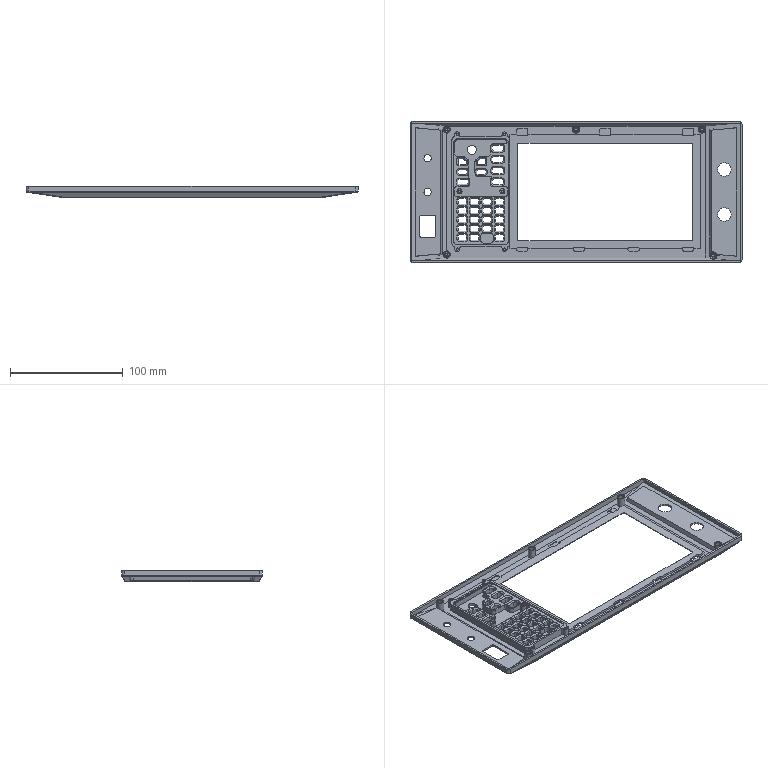NC program | NX | posted with a generic post | part box 295 x 125 x 10 mm
Lines 5491 to 6455 of 134431:
(CAVITY_MILL_COPY , TOOL : D6)
N10944 T06 M6
N10946 G54
N10948 G17 G0 G90 X112.278 Y-56.8 S9500 M3
N10950 G43 Z30. H6
N10952 Z0.5
N10954 G94 G1 Z-0.5 F1000.
N10956 X112.683 Y-57.5
N10958 G3 X113.549 Y-58. R1.
N10960 G1 X115.933 F2000.
N10962 G2 X115.782 Y-55.868 R6.25
N10964 G3 X115.372 Y-54.956 R1.
N10966 G1 X114.81 Y-54.55
N10968 Z0.5
N10970 G0 Z30.
N10972 X112.278 Y-56.8
N10974 Z0.
N10976 G1 Z-1. F1000.
N10978 X112.683 Y-57.5
N10980 G3 X113.549 Y-58. R1.
N10982 G1 X115.933 F2000.
N10984 G2 X115.782 Y-55.869 R6.25
N10986 G3 X115.372 Y-54.956 R1.
N10988 G1 X114.81 Y-54.551
N10990 Z0.
N10992 G0 X112.278 Y-56.8 Z-0.5
N10994 G1 Z-1.5 F1000.
N10996 X112.682 Y-57.5
N10998 G3 X113.548 Y-58. R1.
N11000 G1 X115.933 F2000.
N11002 G2 X115.782 Y-55.869 R6.25
N11004 G3 X115.372 Y-54.956 R1.
N11006 G1 X114.81 Y-54.551
N11008 Z-0.5
N11010 G0 X112.278 Y-56.8 Z-1.
N11012 G1 Z-2. F1000.
N11014 X112.682 Y-57.5
N11016 G3 X113.548 Y-58. R1.
N11018 G1 X115.933 F2000.
N11020 G2 X115.782 Y-55.868 R6.25
N11022 G3 X115.372 Y-54.956 R1.
N11024 G1 X114.81 Y-54.551
N11026 Z-1.
N11028 G0 X112.278 Y-56.8 Z-1.5
N11030 G1 Z-2.5 F1000.
N11032 X112.682 Y-57.5
N11034 G3 X113.548 Y-58. R1.
N11036 G1 X115.933 F2000.
N11038 G2 X115.782 Y-55.868 R6.25
N11040 G3 X115.372 Y-54.956 R1.
N11042 G1 X114.81 Y-54.551
N11044 Z-1.5
N11046 G0 X112.278 Y-56.8 Z-2.
N11048 G1 Z-3. F1000.
N11050 X112.682 Y-57.5
N11052 G3 X113.548 Y-58. R1.
N11054 G1 X115.933 F2000.
N11056 G2 X115.782 Y-55.868 R6.25
N11058 G3 X115.372 Y-54.956 R1.
N11060 G1 X114.81 Y-54.55
N11062 Z-2.
N11064 G0 X112.278 Y-56.8 Z-2.5
N11066 G1 Z-3.5 F1000.
N11068 X112.682 Y-57.5
N11070 G3 X113.548 Y-58. R1.
N11072 G1 X115.933 F2000.
N11074 G2 X115.782 Y-55.868 R6.25
N11076 G3 X115.372 Y-54.956 R1.
N11078 G1 X114.81 Y-54.55
N11080 Z-2.5
N11082 G0 X112.278 Y-56.8 Z-2.885
N11084 G1 Z-3.885 F1000.
N11086 X112.682 Y-57.5
N11088 G3 X113.548 Y-58. R1.
N11090 G1 X115.933 F2000.
N11092 G2 X115.782 Y-55.868 R6.25
N11094 G3 X115.372 Y-54.956 R1.
N11096 G1 X114.81 Y-54.55
N11098 Z-2.885
N11100 G0 X112.278 Y-56.8 Z-3.269
N11102 G1 Z-4.269 F1000.
N11104 X112.682 Y-57.5
N11106 G3 X113.548 Y-58. R1.
N11108 G1 X115.933 F2000.
N11110 G2 X115.782 Y-55.868 R6.25
N11112 G3 X115.372 Y-54.956 R1.
N11114 G1 X114.81 Y-54.55
N11116 Z-3.269
N11118 G0 X112.289 Y-56.655 Z-3.827
N11120 G1 Z-4.827 F1000.
N11122 X112.693 Y-57.355
N11124 G3 X113.559 Y-57.855 R1.
N11126 G1 X115.899 F2000.
N11128 G2 X115.794 Y-55.759 R6.25
N11130 G3 X115.4 Y-54.84 R1.
N11132 G1 X114.845 Y-54.424
N11134 Z-3.827
N11136 G0 X112.322 Y-56.32 Z-4.385
N11138 G1 Z-5.385 F1000.
N11140 X112.726 Y-57.02
N11142 G3 X113.592 Y-57.52 R1.
N11144 G1 X115.834 F2000.
N11146 G2 X115.829 Y-55.507 R6.25
N11148 G3 X115.473 Y-54.572 R1.
N11150 G1 X114.936 Y-54.134
N11152 Z-4.385
N11154 G0 X112.369 Y-55.985 Z-4.942
N11156 G1 Z-5.942 F1000.
N11158 X112.773 Y-56.685
N11160 G3 X113.639 Y-57.185 R1.
N11162 G1 X115.788 F2000.
N11164 G2 X115.875 Y-55.255 R6.25
N11166 G3 X115.558 Y-54.307 R1.
N11168 G1 X114.754 Y-53.595
N11170 Z-4.942
N11172 G0 X112.43 Y-55.652 Z-5.5
N11174 G1 Z-6.5 F1000.
N11176 X112.834 Y-56.352
N11178 G3 X113.7 Y-56.852 R1.
N11180 G1 X115.76 F2000.
N11182 G2 X115.932 Y-55.005 R6.25
N11184 G3 X115.653 Y-54.044 R1.
N11186 G1 X114.743 Y-53.17
N11188 Z-5.5
N11190 G0 X113.114 Y-54.608 Z-6.
N11192 G1 Z-7. F1000.
N11194 X112.113 Y-54.791
N11196 G2 X112.113 Y-53.791 R1.
N11198 X112.421 Y-53.413 R1.52 F2000.
N11200 G3 X112.495 Y-52.746 R0.5
N11202 G2 X110.54 Y-53.47 R3.
N11204 G1 X104.54
N11206 G2 X101.942 Y-51.97 R3.
N11208 G1 X100.753
N11210 G3 X101.183 Y-52.465 R0.5
N11212 G2 X101.933 Y-52.794 R1.52
N11214 G3 X102.545 Y-52.811 R0.5
N11216 X102.659 Y-53.413 R0.5
N11218 G2 X101.864 Y-56.056 R1.52
N11220 G3 X101.434 Y-56.551 R0.5
N11222 G1 X113.646
N11224 G3 X113.216 Y-56.056 R0.5
N11226 G2 X112.113 Y-53.791 R1.52
N11228 X112.979 Y-53.291 R1.
N11230 G1 X113.537 Y-53.931
N11232 Z-6.
N11234 G0 Z30.
N11236 X114.915 Y-54.198
N11238 Z-3.827
N11240 G1 Z-4.827 F1000.
N11242 X115.607 Y-54.166
N11244 G3 X116.45 Y-53.627 R1.
N11246 G2 X116.833 Y-52.983 R6.25 F2000.
N11248 G1 Y-52.197
N11250 G3 X116.333 Y-51.331 R1.
N11252 G1 X115.633 Y-50.927
N11254 Z-3.827
N11256 G0 X114.833 Y-54.467 Z-4.385
N11258 G1 Z-5.385 F1000.
N11260 X115.524 Y-54.409
N11262 G3 X116.345 Y-53.839 R1.
N11264 G2 X116.684 Y-53.214 R6.25 F2000.
N11266 G1 Y-52.471
N11268 G3 X116.184 Y-51.605 R1.
N11270 G1 X115.484 Y-51.201
N11272 Z-4.385
N11274 G0 X114.379 Y-54.809 Z-4.942
N11276 G1 Z-5.942 F1000.
N11278 X115.444 Y-54.675
N11280 G3 X116.241 Y-54.072 R1.
N11282 G2 X116.534 Y-53.469 R6.25 F2000.
N11284 G1 Y-52.773
N11286 G3 X116.034 Y-51.907 R1.
N11288 G1 X115.334 Y-51.502
N11290 Z-4.942
N11292 G0 X113.559 Y-55.278 Z-5.5
N11294 G1 Z-6.5 F1000.
N11296 X115.369 Y-54.969
N11298 G3 X116.139 Y-54.33 R1.
N11300 G2 X116.386 Y-53.754 R6.25 F2000.
N11302 G1 Y-53.108
N11304 G3 X115.886 Y-52.242 R1.
N11306 G1 X115.186 Y-51.838
N11308 Z-5.5
N11310 G0 Z30.
N11312 X129.191 Y-54.551
N11314 Z0.5
N11316 G1 Z-0.5 F1000.
N11318 X128.628 Y-54.957
N11320 G3 X128.218 Y-55.869 R1.
N11322 G2 X128.067 Y-58. R6.25 F2000.
N11324 G1 X130.451
N11326 G3 X131.317 Y-57.5 R1.
N11328 G1 X131.722 Y-56.8
N11330 Z0.5
N11332 G0 Z30.
N11334 X129.19 Y-54.551
N11336 Z0.
N11338 G1 Z-1. F1000.
N11340 X128.628 Y-54.956
N11342 G3 X128.218 Y-55.869 R1.
N11344 G2 X128.067 Y-58. R6.25 F2000.
N11346 G1 X130.452
N11348 G3 X131.318 Y-57.5 R1.
N11350 G1 X131.722 Y-56.8
N11352 Z0.
N11354 G0 X129.19 Y-54.551 Z-0.5
N11356 G1 Z-1.5 F1000.
N11358 X128.628 Y-54.956
N11360 G3 X128.218 Y-55.868 R1.
N11362 G2 X128.067 Y-58. R6.25 F2000.
N11364 G1 X130.452
N11366 G3 X131.318 Y-57.5 R1.
N11368 G1 X131.722 Y-56.8
N11370 Z-0.5
N11372 G0 X129.19 Y-54.551 Z-1.
N11374 G1 Z-2. F1000.
N11376 X128.628 Y-54.956
N11378 G3 X128.218 Y-55.868 R1.
N11380 G2 X128.067 Y-58. R6.25 F2000.
N11382 G1 X130.452
N11384 G3 X131.318 Y-57.5 R1.
N11386 G1 X131.722 Y-56.8
N11388 Z-1.
N11390 G0 X129.19 Y-54.55 Z-1.5
N11392 G1 Z-2.5 F1000.
N11394 X128.628 Y-54.956
N11396 G3 X128.218 Y-55.868 R1.
N11398 G2 X128.067 Y-58. R6.25 F2000.
N11400 G1 X130.452
N11402 G3 X131.318 Y-57.5 R1.
N11404 G1 X131.722 Y-56.8
N11406 Z-1.5
N11408 G0 X129.19 Y-54.55 Z-2.
N11410 G1 Z-3. F1000.
N11412 X128.628 Y-54.956
N11414 G3 X128.218 Y-55.868 R1.
N11416 G2 X128.067 Y-58. R6.25 F2000.
N11418 G1 X130.452
N11420 G3 X131.318 Y-57.5 R1.
N11422 G1 X131.722 Y-56.8
N11424 Z-2.
N11426 G0 X129.19 Y-54.55 Z-2.5
N11428 G1 Z-3.5 F1000.
N11430 X128.628 Y-54.956
N11432 G3 X128.218 Y-55.868 R1.
N11434 G2 X128.067 Y-58. R6.25 F2000.
N11436 G1 X130.452
N11438 G3 X131.318 Y-57.5 R1.
N11440 G1 X131.722 Y-56.8
N11442 Z-2.5
N11444 G0 X129.19 Y-54.55 Z-2.885
N11446 G1 Z-3.885 F1000.
N11448 X128.628 Y-54.956
N11450 G3 X128.218 Y-55.868 R1.
N11452 G2 X128.067 Y-58. R6.25 F2000.
N11454 G1 X130.452
N11456 G3 X131.318 Y-57.5 R1.
N11458 G1 X131.722 Y-56.8
N11460 Z-2.885
N11462 G0 X129.19 Y-54.55 Z-3.269
N11464 G1 Z-4.269 F1000.
N11466 X128.628 Y-54.956
N11468 G3 X128.218 Y-55.868 R1.
N11470 G2 X128.067 Y-58. R6.25 F2000.
N11472 G1 X130.452
N11474 G3 X131.318 Y-57.5 R1.
N11476 G1 X131.722 Y-56.8
N11478 Z-3.269
N11480 G0 Z30.
N11482 X139.513
N11484 Z0.5
N11486 G1 Z-0.5 F1000.
N11488 X139.918 Y-57.5
N11490 G3 X140.784 Y-58. R1.
N11492 G1 X143. F2000.
N11494 Y-55.784
N11496 G3 X142.5 Y-54.918 R1.
N11498 G1 X141.8 Y-54.513
N11500 Z0.5
N11502 G0 Z30.
N11504 X139.513 Y-56.8
N11506 Z0.
N11508 G1 Z-1. F1000.
N11510 X139.918 Y-57.5
N11512 G3 X140.784 Y-58. R1.
N11514 G1 X143. F2000.
N11516 Y-55.784
N11518 G3 X142.5 Y-54.918 R1.
N11520 G1 X141.8 Y-54.513
N11522 Z0.
N11524 G0 X139.513 Y-56.8 Z-0.5
N11526 G1 Z-1.5 F1000.
N11528 X139.918 Y-57.5
N11530 G3 X140.784 Y-58. R1.
N11532 G1 X143. F2000.
N11534 Y-55.784
N11536 G3 X142.5 Y-54.918 R1.
N11538 G1 X141.8 Y-54.513
N11540 Z-0.5
N11542 G0 X139.513 Y-56.8 Z-1.
N11544 G1 Z-2. F1000.
N11546 X139.918 Y-57.5
N11548 G3 X140.784 Y-58. R1.
N11550 G1 X143. F2000.
N11552 Y-55.784
N11554 G3 X142.5 Y-54.918 R1.
N11556 G1 X141.8 Y-54.513
N11558 Z-1.
N11560 G0 X139.513 Y-56.8 Z-1.5
N11562 G1 Z-2.5 F1000.
N11564 X139.918 Y-57.5
N11566 G3 X140.784 Y-58. R1.
N11568 G1 X143. F2000.
N11570 Y-55.784
N11572 G3 X142.5 Y-54.918 R1.
N11574 G1 X141.8 Y-54.513
N11576 Z-1.5
N11578 G0 X139.513 Y-56.8 Z-2.
N11580 G1 Z-3. F1000.
N11582 X139.918 Y-57.5
N11584 G3 X140.784 Y-58. R1.
N11586 G1 X143. F2000.
N11588 Y-55.784
N11590 G3 X142.5 Y-54.918 R1.
N11592 G1 X141.8 Y-54.513
N11594 Z-2.
N11596 G0 X139.513 Y-56.8 Z-2.5
N11598 G1 Z-3.5 F1000.
N11600 X139.918 Y-57.5
N11602 G3 X140.784 Y-58. R1.
N11604 G1 X143. F2000.
N11606 Y-55.784
N11608 G3 X142.5 Y-54.918 R1.
N11610 G1 X141.8 Y-54.513
N11612 Z-2.5
N11614 G0 X138.399 Y-56.8 Z-2.885
N11616 G1 Z-3.885 F1000.
N11618 X138.803 Y-57.5
N11620 G3 X139.669 Y-58. R1.
N11622 G1 X141.885 F2000.
N11624 Y-55.784
N11626 G3 X141.385 Y-54.918 R1.
N11628 G1 X140.685 Y-54.513
N11630 Z-2.885
N11632 G0 X135.915 Y-56.8 Z-3.269
N11634 G1 Z-4.269 F1000.
N11636 X136.319 Y-57.5
N11638 G3 X137.185 Y-58. R1.
N11640 G1 X139.402 F2000.
N11642 Y-55.784
N11644 G3 X138.902 Y-54.918 R1.
N11646 G1 X138.202 Y-54.513
N11648 Z-3.269
N11650 G0 Z30.
N11652 X97.053 Y-39.27
N11654 Z-6.
N11656 G1 Z-7. F1000.
N11658 X97.458 Y-39.97
N11660 G3 X98.324 Y-40.47 R1.
N11662 G1 X100.54 F2000.
N11664 Y-38.254
N11666 G3 X100.04 Y-37.388 R1.
N11668 G1 X99.34 Y-36.983
N11670 Z-6.
N11672 G0 X97.044 Y-39.27 Z-6.5
N11674 G1 Z-7.5 F1000.
N11676 X97.448 Y-39.97
N11678 G3 X98.314 Y-40.47 R1.
N11680 G1 X100.54 F2000.
N11682 Y-38.253
N11684 G3 X100.04 Y-37.387 R1.
N11686 G1 X99.34 Y-36.983
N11688 Z-6.5
N11690 G0 X97.044 Y-39.27 Z-7.
N11692 G1 Z-8. F1000.
N11694 X97.448 Y-39.97
N11696 G3 X98.314 Y-40.47 R1.
N11698 G1 X100.54 F2000.
N11700 Y-38.253
N11702 G3 X100.04 Y-37.387 R1.
N11704 G1 X99.34 Y-36.983
N11706 Z-7.
N11708 G0 X97.044 Y-39.27 Z-7.5
N11710 G1 Z-8.5 F1000.
N11712 X97.448 Y-39.97
N11714 G3 X98.314 Y-40.47 R1.
N11716 G1 X100.54 F2000.
N11718 Y-38.253
N11720 G3 X100.04 Y-37.387 R1.
N11722 G1 X99.34 Y-36.983
N11724 Z-7.5
N11726 G0 X97.044 Y-39.27 Z-7.85
N11728 G1 Z-8.85 F1000.
N11730 X97.448 Y-39.97
N11732 G3 X98.314 Y-40.47 R1.
N11734 G1 X100.54 F2000.
N11736 Y-38.253
N11738 G3 X100.04 Y-37.387 R1.
N11740 G1 X99.34 Y-36.983
N11742 Z-7.85
N11744 G0 X97.044 Y-39.27 Z-8.2
N11746 G1 Z-9.2 F1000.
N11748 X97.448 Y-39.97
N11750 G3 X98.314 Y-40.47 R1.
N11752 G1 X100.54 F2000.
N11754 Y-38.253
N11756 G3 X100.04 Y-37.387 R1.
N11758 G1 X99.34 Y-36.983
N11760 Z-8.2
N11762 G0 X97.044 Y-39.27 Z-8.6
N11764 G1 Z-9.6 F1000.
N11766 X97.448 Y-39.97
N11768 G3 X98.314 Y-40.47 R1.
N11770 G1 X100.54 F2000.
N11772 Y-38.253
N11774 G3 X100.04 Y-37.387 R1.
N11776 G1 X99.34 Y-36.983
N11778 Z-8.6
N11780 G0 X97.044 Y-39.27 Z-9.
N11782 G1 Z-10. F1000.
N11784 X97.448 Y-39.97
N11786 G3 X98.314 Y-40.47 R1.
N11788 G1 X100.54 F2000.
N11790 Y-38.253
N11792 G3 X100.04 Y-37.387 R1.
N11794 G1 X99.34 Y-36.983
N11796 Z-9.
N11798 G0 Z30.
N11800 Y36.963
N11802 Z-6.
N11804 G1 Z-7. F1000.
N11806 X100.04 Y37.368
N11808 G3 X100.54 Y38.234 R1.
N11810 G1 Y40.45 F2000.
N11812 X98.324
N11814 G3 X97.458 Y39.95 R1.
N11816 G1 X97.053 Y39.25
N11818 Z-6.
N11820 G0 X99.34 Y36.97 Z-6.5
N11822 G1 Z-7.5 F1000.
N11824 X100.04 Y37.374
N11826 G3 X100.54 Y38.24 R1.
N11828 G1 Y40.45 F2000.
N11830 X98.33
N11832 G3 X97.464 Y39.95 R1.
N11834 G1 X97.06 Y39.25
N11836 Z-6.5
N11838 G0 X99.34 Y36.97 Z-7.
N11840 G1 Z-8. F1000.
N11842 X100.04 Y37.374
N11844 G3 X100.54 Y38.24 R1.
N11846 G1 Y40.45 F2000.
N11848 X98.33
N11850 G3 X97.464 Y39.95 R1.
N11852 G1 X97.06 Y39.25
N11854 Z-7.
N11856 G0 X99.34 Y36.97 Z-7.5
N11858 G1 Z-8.5 F1000.
N11860 X100.04 Y37.374
N11862 G3 X100.54 Y38.24 R1.
N11864 G1 Y40.45 F2000.
N11866 X98.33
N11868 G3 X97.464 Y39.95 R1.
N11870 G1 X97.06 Y39.25
N11872 Z-7.5
N11874 G0 X99.34 Y36.97 Z-7.85
N11876 G1 Z-8.85 F1000.
N11878 X100.04 Y37.374
N11880 G3 X100.54 Y38.24 R1.
N11882 G1 Y40.45 F2000.
N11884 X98.33
N11886 G3 X97.464 Y39.95 R1.
N11888 G1 X97.06 Y39.25
N11890 Z-7.85
N11892 G0 X99.34 Y36.97 Z-8.2
N11894 G1 Z-9.2 F1000.
N11896 X100.04 Y37.374
N11898 G3 X100.54 Y38.24 R1.
N11900 G1 Y40.45 F2000.
N11902 X98.33
N11904 G3 X97.464 Y39.95 R1.
N11906 G1 X97.06 Y39.25
N11908 Z-8.2
N11910 G0 X99.34 Y36.97 Z-8.6
N11912 G1 Z-9.6 F1000.
N11914 X100.04 Y37.374
N11916 G3 X100.54 Y38.24 R1.
N11918 G1 Y40.45 F2000.
N11920 X98.33
N11922 G3 X97.464 Y39.95 R1.
N11924 G1 X97.06 Y39.25
N11926 Z-8.6
N11928 G0 X99.34 Y36.97 Z-9.
N11930 G1 Z-10. F1000.
N11932 X100.04 Y37.374
N11934 G3 X100.54 Y38.24 R1.
N11936 G1 Y40.45 F2000.
N11938 X98.33
N11940 G3 X97.464 Y39.95 R1.
N11942 G1 X97.06 Y39.25
N11944 Z-9.
N11946 G0 Z30.
N11948 X141.8 Y54.513
N11950 Z0.5
N11952 G1 Z-0.5 F1000.
N11954 X142.5 Y54.918
N11956 G3 X143. Y55.784 R1.
N11958 G1 Y58. F2000.
N11960 X140.784
N11962 G3 X139.918 Y57.5 R1.
N11964 G1 X139.513 Y56.8
N11966 Z0.5
N11968 G0 Z30.
N11970 X141.8 Y54.513
N11972 Z0.
N11974 G1 Z-1. F1000.
N11976 X142.5 Y54.918
N11978 G3 X143. Y55.784 R1.
N11980 G1 Y58. F2000.
N11982 X140.784
N11984 G3 X139.918 Y57.5 R1.
N11986 G1 X139.513 Y56.8
N11988 Z0.
N11990 G0 X141.8 Y54.513 Z-0.5
N11992 G1 Z-1.5 F1000.
N11994 X142.5 Y54.918
N11996 G3 X143. Y55.784 R1.
N11998 G1 Y58. F2000.
N12000 X140.784
N12002 G3 X139.918 Y57.5 R1.
N12004 G1 X139.513 Y56.8
N12006 Z-0.5
N12008 G0 X141.8 Y54.513 Z-1.
N12010 G1 Z-2. F1000.
N12012 X142.5 Y54.918
N12014 G3 X143. Y55.784 R1.
N12016 G1 Y58. F2000.
N12018 X140.784
N12020 G3 X139.918 Y57.5 R1.
N12022 G1 X139.513 Y56.8
N12024 Z-1.
N12026 G0 X141.8 Y54.513 Z-1.5
N12028 G1 Z-2.5 F1000.
N12030 X142.5 Y54.918
N12032 G3 X143. Y55.784 R1.
N12034 G1 Y58. F2000.
N12036 X140.784
N12038 G3 X139.918 Y57.5 R1.
N12040 G1 X139.513 Y56.8
N12042 Z-1.5
N12044 G0 X141.8 Y54.513 Z-2.
N12046 G1 Z-3. F1000.
N12048 X142.5 Y54.918
N12050 G3 X143. Y55.784 R1.
N12052 G1 Y58. F2000.
N12054 X140.784
N12056 G3 X139.918 Y57.5 R1.
N12058 G1 X139.513 Y56.8
N12060 Z-2.
N12062 G0 X141.8 Y54.513 Z-2.5
N12064 G1 Z-3.5 F1000.
N12066 X142.5 Y54.918
N12068 G3 X143. Y55.784 R1.
N12070 G1 Y58. F2000.
N12072 X140.784
N12074 G3 X139.918 Y57.5 R1.
N12076 G1 X139.513 Y56.8
N12078 Z-2.5
N12080 G0 X140.685 Y54.513 Z-2.885
N12082 G1 Z-3.885 F1000.
N12084 X141.385 Y54.918
N12086 G3 X141.885 Y55.784 R1.
N12088 G1 Y58. F2000.
N12090 X139.669
N12092 G3 X138.803 Y57.5 R1.
N12094 G1 X138.399 Y56.8
N12096 Z-2.885
N12098 G0 X138.202 Y54.513 Z-3.269
N12100 G1 Z-4.269 F1000.
N12102 X138.902 Y54.918
N12104 G3 X139.402 Y55.784 R1.
N12106 G1 Y58. F2000.
N12108 X137.185
N12110 G3 X136.319 Y57.5 R1.
N12112 G1 X135.915 Y56.8
N12114 Z-3.269
N12116 G0 Z30.
N12118 X121.721
N12120 Z0.5
N12122 G1 Z-0.5 F1000.
N12124 X121.317 Y57.5
N12126 G3 X120.451 Y58. R1.
N12128 G1 X117.728 F2000.
N12130 G2 X118.249 Y55.626 R6.25
N12132 G3 X118.766 Y54.77 R1.
N12134 G1 X119.374 Y54.435
N12136 Z0.5
N12138 G0 Z30.
N12140 X121.721 Y56.8
N12142 Z0.
N12144 G1 Z-1. F1000.
N12146 X121.317 Y57.5
N12148 G3 X120.451 Y58. R1.
N12150 G1 X117.728 F2000.
N12152 G2 X118.249 Y55.626 R6.25
N12154 G3 X118.766 Y54.77 R1.
N12156 G1 X119.374 Y54.435
N12158 Z0.
N12160 G0 X121.721 Y56.8 Z-0.5
N12162 G1 Z-1.5 F1000.
N12164 X121.317 Y57.5
N12166 G3 X120.451 Y58. R1.
N12168 G1 X117.728 F2000.
N12170 G2 X118.249 Y55.626 R6.25
N12172 G3 X118.766 Y54.77 R1.
N12174 G1 X119.374 Y54.435
N12176 Z-0.5
N12178 G0 X121.721 Y56.8 Z-1.
N12180 G1 Z-2. F1000.
N12182 X121.317 Y57.5
N12184 G3 X120.451 Y58. R1.
N12186 G1 X117.728 F2000.
N12188 G2 X118.249 Y55.626 R6.25
N12190 G3 X118.766 Y54.77 R1.
N12192 G1 X119.374 Y54.435
N12194 Z-1.
N12196 G0 X121.721 Y56.8 Z-1.5
N12198 G1 Z-2.5 F1000.
N12200 X121.317 Y57.5
N12202 G3 X120.451 Y58. R1.
N12204 G1 X117.728 F2000.
N12206 G2 X118.249 Y55.626 R6.25
N12208 G3 X118.766 Y54.77 R1.
N12210 G1 X119.374 Y54.435
N12212 Z-1.5
N12214 G0 X121.721 Y56.8 Z-2.
N12216 G1 Z-3. F1000.
N12218 X121.317 Y57.5
N12220 G3 X120.451 Y58. R1.
N12222 G1 X117.728 F2000.
N12224 G2 X118.249 Y55.626 R6.25
N12226 G3 X118.766 Y54.77 R1.
N12228 G1 X119.374 Y54.435
N12230 Z-2.
N12232 G0 X121.721 Y56.8 Z-2.5
N12234 G1 Z-3.5 F1000.
N12236 X121.317 Y57.5
N12238 G3 X120.451 Y58. R1.
N12240 G1 X117.728 F2000.
N12242 G2 X118.249 Y55.626 R6.25
N12244 G3 X118.766 Y54.77 R1.
N12246 G1 X119.374 Y54.435
N12248 Z-2.5
N12250 G0 X121.721 Y56.8 Z-2.885
N12252 G1 Z-3.885 F1000.
N12254 X121.317 Y57.5
N12256 G3 X120.451 Y58. R1.
N12258 G1 X117.728 F2000.
N12260 G2 X118.249 Y55.626 R6.25
N12262 G3 X118.766 Y54.77 R1.
N12264 G1 X119.374 Y54.435
N12266 Z-2.885
N12268 G0 X121.721 Y56.8 Z-3.269
N12270 G1 Z-4.269 F1000.
N12272 X121.317 Y57.5
N12274 G3 X120.451 Y58. R1.
N12276 G1 X117.728 F2000.
N12278 G2 X118.249 Y55.626 R6.25
N12280 G3 X118.766 Y54.77 R1.
N12282 G1 X119.374 Y54.435
N12284 Z-3.269
N12286 G0 X115.633 Y46.265 Z-3.827
N12288 G1 Z-4.827 F1000.
N12290 X116.333 Y46.669
N12292 G3 X116.833 Y47.535 R1.
N12294 G1 Y51.537 F2000.
N12296 G2 X113.907 Y49.548 R6.25
N12298 G3 X113.235 Y48.808 R1.
N12300 G1 X113.088 Y48.13
N12302 Z-3.827
N12304 G0 X115.484 Y46.212 Z-4.385
N12306 G1 Z-5.385 F1000.
N12308 X116.184 Y46.616
N12310 G3 X116.684 Y47.482 R1.
N12312 G1 Y51.362 F2000.
N12314 G2 X113.792 Y49.512 R6.25
N12316 G3 X113.106 Y48.785 R1.
N12318 G1 X112.946 Y48.11
N12320 Z-4.385
N12322 G0 X115.334 Y46.162 Z-4.942
N12324 G1 Z-5.942 F1000.
N12326 X116.034 Y46.566
N12328 G3 X116.534 Y47.432 R1.
N12330 G1 Y51.199 F2000.
N12332 G2 X113.677 Y49.479 R6.25
N12334 G3 X112.977 Y48.765 R1.
N12336 G1 X112.804 Y48.094
N12338 Z-4.942
N12340 G0 X115.186 Y46.116 Z-5.5
N12342 G1 Z-6.5 F1000.
N12344 X115.886 Y46.52
N12346 G3 X116.386 Y47.386 R1.
N12348 G1 Y51.047 F2000.
N12350 G2 X113.563 Y49.449 R6.25
N12352 G3 X112.85 Y48.748 R1.
N12354 G1 X112.664 Y48.08
N12356 Z-5.5
N12358 G0 X113.323 Y-54.853 Z-6.
N12360 G1 Z-7. F1000.
N12362 X112.901 Y-56.051
N12364 G3 X113.767 Y-56.551 R1.
N12366 G1 X115.75 F2000.
N12368 Y-56.493
N12370 G2 X116.251 Y-54.048 R6.25
N12372 G1 Y50.918
N12374 G2 X113.54 Y49.443 R6.25
N12376 G1 Y-50.47
N12378 G2 X112.513 Y-52.73 R3.
N12380 G3 X112.19 Y-53.676 R1.
N12382 G1 X113.168 Y-54.366
N12384 Z-6.
N12386 G0 X113.497 Y-54.319 Z-6.5
N12388 G1 Z-7.5 F1000.
N12390 X112.501 Y-54.53
N12392 G2 X112.472 Y-53.531 R1.
N12394 G1 X111.888 Y-53.317
N12396 X111.824 Y-53.181
N12398 G2 X110.54 Y-53.47 R3. F2000.
N12400 G1 X104.54
N12402 G2 X101.942 Y-51.97 R3.
N12404 G1 X100.753
N12406 G3 X101.183 Y-52.465 R0.5
N12408 G2 X101.933 Y-52.794 R1.52
N12410 G3 X102.25 Y-52.908 R0.5
N12412 X102.383 Y-53.217 R0.5
N12414 G2 X101.483 Y-55.757 R1.52
N12416 G3 X101.053 Y-56.252 R0.5
N12418 G1 X115.755
N12420 G2 X116.118 Y-54.388 R6.25
N12422 G1 Y50.798
N12424 G2 X113.54 Y49.443 R6.25
N12426 G1 Y-50.47
N12428 G2 X111.824 Y-53.181 R3.
N12430 G3 X111.256 Y-54.004 R1.
N12432 G1 X113.492 Y-54.221
N12434 Z-6.5
N12436 G0 Z30.
N12438 X104.626 Y54.435
N12440 Z0.5
N12442 G1 Z-0.5 F1000.
N12444 X105.234 Y54.77
N12446 G3 X105.751 Y55.626 R1.
N12448 G2 X106.272 Y58. R6.25 F2000.
N12450 G1 X103.549
N12452 G3 X102.683 Y57.5 R1.
N12454 G1 X102.279 Y56.8
N12456 Z0.5
N12458 G0 Z30.
N12460 X104.626 Y54.435
N12462 Z0.
N12464 G1 Z-1. F1000.
N12466 X105.234 Y54.77
N12468 G3 X105.751 Y55.626 R1.
N12470 G2 X106.272 Y58. R6.25 F2000.
N12472 G1 X103.549
N12474 G3 X102.683 Y57.5 R1.
N12476 G1 X102.279 Y56.8
N12478 Z0.
N12480 G0 X104.626 Y54.435 Z-0.5
N12482 G1 Z-1.5 F1000.
N12484 X105.234 Y54.77
N12486 G3 X105.751 Y55.626 R1.
N12488 G2 X106.272 Y58. R6.25 F2000.
N12490 G1 X103.549
N12492 G3 X102.683 Y57.5 R1.
N12494 G1 X102.279 Y56.8
N12496 Z-0.5
N12498 G0 X104.626 Y54.435 Z-1.
N12500 G1 Z-2. F1000.
N12502 X105.234 Y54.77
N12504 G3 X105.751 Y55.626 R1.
N12506 G2 X106.272 Y58. R6.25 F2000.
N12508 G1 X103.549
N12510 G3 X102.683 Y57.5 R1.
N12512 G1 X102.279 Y56.8
N12514 Z-1.
N12516 G0 X104.626 Y54.435 Z-1.5
N12518 G1 Z-2.5 F1000.
N12520 X105.234 Y54.77
N12522 G3 X105.751 Y55.626 R1.
N12524 G2 X106.272 Y58. R6.25 F2000.
N12526 G1 X103.549
N12528 G3 X102.683 Y57.5 R1.
N12530 G1 X102.279 Y56.8
N12532 Z-1.5
N12534 G0 X104.626 Y54.435 Z-2.
N12536 G1 Z-3. F1000.
N12538 X105.234 Y54.77
N12540 G3 X105.751 Y55.626 R1.
N12542 G2 X106.272 Y58. R6.25 F2000.
N12544 G1 X103.549
N12546 G3 X102.683 Y57.5 R1.
N12548 G1 X102.279 Y56.8
N12550 Z-2.
N12552 G0 X104.626 Y54.435 Z-2.5
N12554 G1 Z-3.5 F1000.
N12556 X105.234 Y54.77
N12558 G3 X105.751 Y55.626 R1.
N12560 G2 X106.272 Y58. R6.25 F2000.
N12562 G1 X103.549
N12564 G3 X102.683 Y57.5 R1.
N12566 G1 X102.279 Y56.8
N12568 Z-2.5
N12570 G0 X104.626 Y54.435 Z-2.885
N12572 G1 Z-3.885 F1000.
N12574 X105.234 Y54.77
N12576 G3 X105.751 Y55.626 R1.
N12578 G2 X106.272 Y58. R6.25 F2000.
N12580 G1 X103.549
N12582 G3 X102.683 Y57.5 R1.
N12584 G1 X102.279 Y56.8
N12586 Z-2.885
N12588 G0 X104.626 Y54.435 Z-3.269
N12590 G1 Z-4.269 F1000.
N12592 X105.234 Y54.77
N12594 G3 X105.751 Y55.626 R1.
N12596 G2 X106.272 Y58. R6.25 F2000.
N12598 G1 X103.549
N12600 G3 X102.683 Y57.5 R1.
N12602 G1 X102.279 Y56.8
N12604 Z-3.269
N12606 G0 X104.646 Y54.305 Z-3.827
N12608 G1 Z-4.827 F1000.
N12610 X105.248 Y54.651
N12612 G3 X105.75 Y55.515 R1.
N12614 G2 X106.21 Y57.855 R6.25 F2000.
N12616 G1 X103.541
N12618 G3 X102.675 Y57.355 R1.
N12620 G1 X102.271 Y56.655
N12622 Z-3.827
N12624 G0 X104.701 Y54.008 Z-4.385
N12626 G1 Z-5.385 F1000.
N12628 X105.288 Y54.377
N12630 G3 X105.755 Y55.262 R1.
N12632 G2 X106.085 Y57.52 R6.25 F2000.
N12634 G1 X103.534
N12636 G3 X102.668 Y57.02 R1.
N12638 G1 X102.263 Y56.32
N12640 Z-4.385
N12642 G0 X104.767 Y53.713 Z-4.942
N12644 G1 Z-5.942 F1000.
N12646 X105.339 Y54.106
N12648 G3 X105.769 Y55.009 R1.
N12650 G2 X105.982 Y57.185 R6.25 F2000.
N12652 G1 X103.54
N12654 G3 X102.674 Y56.685 R1.
N12656 G1 X102.269 Y55.985
N12658 Z-4.942
N12660 G0 X104.846 Y53.422 Z-5.5
N12662 G1 Z-6.5 F1000.
N12664 X105.401 Y53.838
N12666 G3 X105.794 Y54.757 R1.
N12668 G2 X105.898 Y56.852 R6.25 F2000.
N12670 G1 X103.559
N12672 G3 X102.693 Y56.352 R1.
N12674 G1 X102.289 Y55.652
N12676 Z-5.5
N12678 G0 Z30.
N12680 X9.721 Y56.8
N12682 Z0.5
N12684 G1 Z-0.5 F1000.
N12686 X9.317 Y57.5
N12688 G3 X8.451 Y58. R1.
N12690 G1 X5.728 F2000.
N12692 G2 X6.249 Y55.626 R6.25
N12694 G3 X6.766 Y54.77 R1.
N12696 G1 X7.374 Y54.435
N12698 Z0.5
N12700 G0 Z30.
N12702 X9.721 Y56.8
N12704 Z0.
N12706 G1 Z-1. F1000.
N12708 X9.317 Y57.5
N12710 G3 X8.451 Y58. R1.
N12712 G1 X5.728 F2000.
N12714 G2 X6.249 Y55.626 R6.25
N12716 G3 X6.766 Y54.77 R1.
N12718 G1 X7.374 Y54.435
N12720 Z0.
N12722 G0 X9.721 Y56.8 Z-0.5
N12724 G1 Z-1.5 F1000.
N12726 X9.317 Y57.5
N12728 G3 X8.451 Y58. R1.
N12730 G1 X5.728 F2000.
N12732 G2 X6.249 Y55.626 R6.25
N12734 G3 X6.766 Y54.77 R1.
N12736 G1 X7.374 Y54.435
N12738 Z-0.5
N12740 G0 X9.721 Y56.8 Z-1.
N12742 G1 Z-2. F1000.
N12744 X9.317 Y57.5
N12746 G3 X8.451 Y58. R1.
N12748 G1 X5.728 F2000.
N12750 G2 X6.249 Y55.626 R6.25
N12752 G3 X6.766 Y54.77 R1.
N12754 G1 X7.374 Y54.435
N12756 Z-1.
N12758 G0 X9.721 Y56.8 Z-1.5
N12760 G1 Z-2.5 F1000.
N12762 X9.317 Y57.5
N12764 G3 X8.451 Y58. R1.
N12766 G1 X5.728 F2000.
N12768 G2 X6.249 Y55.626 R6.25
N12770 G3 X6.766 Y54.77 R1.
N12772 G1 X7.374 Y54.435
N12774 Z-1.5
N12776 G0 X9.721 Y56.8 Z-2.
N12778 G1 Z-3. F1000.
N12780 X9.317 Y57.5
N12782 G3 X8.451 Y58. R1.
N12784 G1 X5.728 F2000.
N12786 G2 X6.249 Y55.626 R6.25
N12788 G3 X6.766 Y54.77 R1.
N12790 G1 X7.374 Y54.435
N12792 Z-2.
N12794 G0 X9.721 Y56.8 Z-2.5
N12796 G1 Z-3.5 F1000.
N12798 X9.317 Y57.5
N12800 G3 X8.451 Y58. R1.
N12802 G1 X5.728 F2000.
N12804 G2 X6.249 Y55.626 R6.25
N12806 G3 X6.766 Y54.77 R1.
N12808 G1 X7.374 Y54.435
N12810 Z-2.5
N12812 G0 X9.721 Y56.8 Z-2.885
N12814 G1 Z-3.885 F1000.
N12816 X9.317 Y57.5
N12818 G3 X8.451 Y58. R1.
N12820 G1 X5.728 F2000.
N12822 G2 X6.249 Y55.626 R6.25
N12824 G3 X6.766 Y54.77 R1.
N12826 G1 X7.374 Y54.435
N12828 Z-2.885
N12830 G0 X9.721 Y56.8 Z-3.269
N12832 G1 Z-4.269 F1000.
N12834 X9.317 Y57.5
N12836 G3 X8.451 Y58. R1.
N12838 G1 X5.728 F2000.
N12840 G2 X6.249 Y55.626 R6.25
N12842 G3 X6.766 Y54.77 R1.
N12844 G1 X7.374 Y54.435
N12846 Z-3.269
N12848 G0 X9.729 Y56.655 Z-3.827
N12850 G1 Z-4.827 F1000.
N12852 X9.325 Y57.355
N12854 G3 X8.459 Y57.855 R1.
N12856 G1 X5.79 F2000.
N12858 G2 X6.25 Y55.515 R6.25
N12860 G3 X6.752 Y54.651 R1.
N12862 G1 X7.354 Y54.305
N12864 Z-3.827
N12866 G0 X9.737 Y56.32 Z-4.385